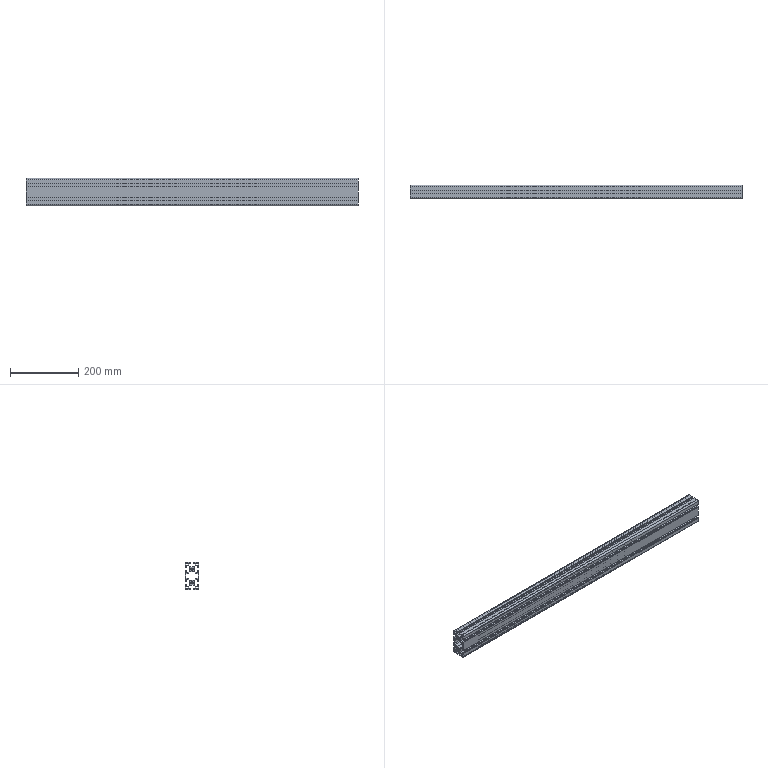Part | SolidWorks | features BaseBody 1 | 1 solid | 130 faces | box 975 x 40 x 80 mm | volume 1189517 mm3 | plane 118 | cylinder 12 | commonest cylinder face diameters 5 x4 6.8 x4 9 x4